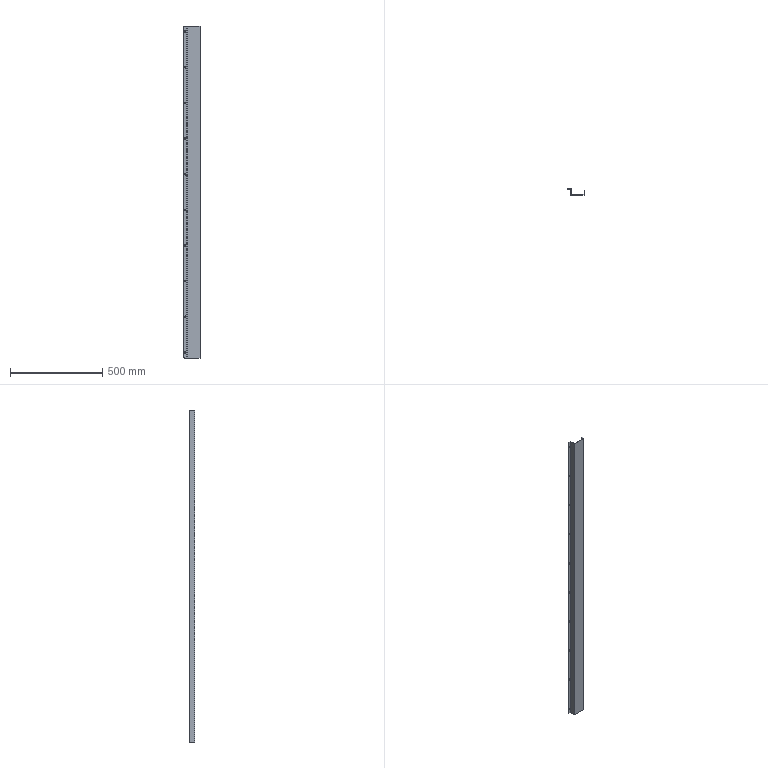Part | SolidWorks | features Fillet 1, FlatPattern 1, ICE 1, SMBaseFlange 1, SheetMetal 1 | 1 solid | 84 faces | box 92 x 32 x 1800 mm | volume 504480 mm3 | plane 44 | cylinder 40 | commonest cylinder face diameters 4 x30 10 x4 0.6 x3 4.6 x3